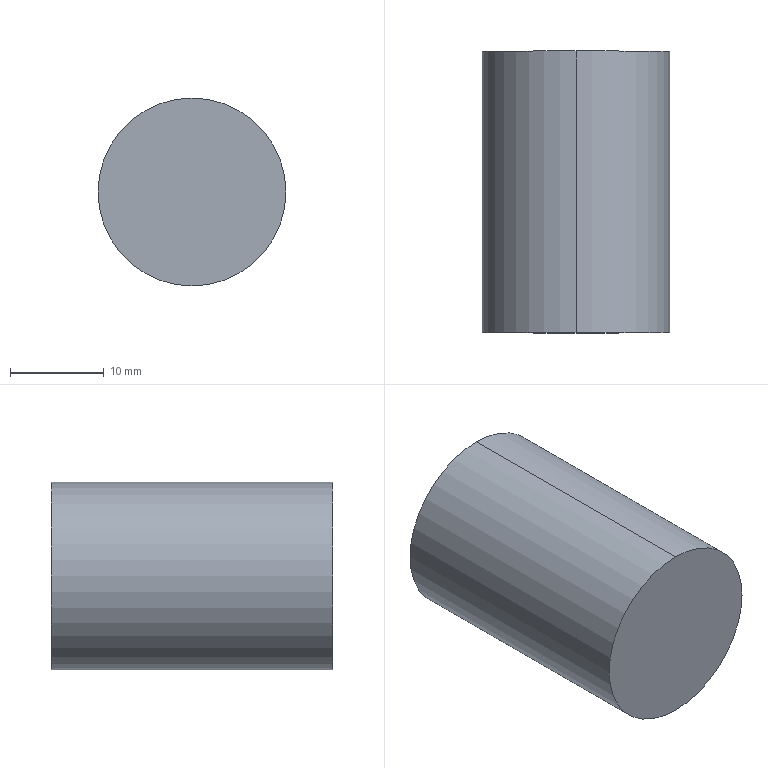Part | SolidWorks | features Extrusion 1 | 1 solid | 4 faces | box 20 x 30 x 20 mm | volume 9425 mm3 | cylinder 2 | plane 2 | commonest cylinder face diameters 20 x2
STEP:
#1=CARTESIAN_POINT('',(0.,30.,10.));
#2=VERTEX_POINT('',#1);
#3=CARTESIAN_POINT('',(0.,30.,-10.));
#4=VERTEX_POINT('',#3);
#5=CARTESIAN_POINT('',(0.,30.,0.));
#6=DIRECTION('',(0.,1.,0.));
#7=DIRECTION('',(0.,0.,1.));
#8=AXIS2_PLACEMENT_3D('',#5,#6,#7);
#9=CIRCLE('',#8,10.);
#10=EDGE_CURVE('',#2,#4,#9,.T.);
#11=ORIENTED_EDGE('',*,*,#10,.F.);
#12=CARTESIAN_POINT('',(0.,0.,10.));
#13=VERTEX_POINT('',#12);
#14=CARTESIAN_POINT('',(0.,30.,10.));
#15=DIRECTION('',(0.,-1.,0.));
#16=VECTOR('',#15,1000.);
#17=LINE('',#14,#16);
#18=EDGE_CURVE('',#2,#13,#17,.T.);
#19=ORIENTED_EDGE('',*,*,#18,.T.);
#20=CARTESIAN_POINT('',(0.,0.,-10.));
#21=VERTEX_POINT('',#20);
#22=CARTESIAN_POINT('',(0.,0.,0.));
#23=DIRECTION('',(0.,1.,0.));
#24=DIRECTION('',(0.,0.,1.));
#25=AXIS2_PLACEMENT_3D('',#22,#23,#24);
#26=CIRCLE('',#25,10.);
#27=EDGE_CURVE('',#13,#21,#26,.T.);
#28=ORIENTED_EDGE('',*,*,#27,.T.);
#29=CARTESIAN_POINT('',(0.,30.,-10.));
#30=DIRECTION('',(0.,-1.,0.));
#31=VECTOR('',#30,1000.);
#32=LINE('',#29,#31);
#33=EDGE_CURVE('',#4,#21,#32,.T.);
#34=ORIENTED_EDGE('',*,*,#33,.F.);
#35=EDGE_LOOP('',(#11,#19,#28,#34));
#36=FACE_OUTER_BOUND('',#35,.T.);
#37=CARTESIAN_POINT('',(0.,30.,0.));
#38=DIRECTION('',(0.,-1.,0.));
#39=DIRECTION('',(0.,0.,-1.));
#40=AXIS2_PLACEMENT_3D('',#37,#38,#39);
#41=CYLINDRICAL_SURFACE('',#40,10.);
#42=ADVANCED_FACE('',(#36),#41,.T.);
#43=ORIENTED_EDGE('',*,*,#18,.F.);
#44=CARTESIAN_POINT('',(0.,30.,0.));
#45=DIRECTION('',(0.,1.,0.));
#46=DIRECTION('',(0.,0.,1.));
#47=AXIS2_PLACEMENT_3D('',#44,#45,#46);
#48=CIRCLE('',#47,10.);
#49=EDGE_CURVE('',#4,#2,#48,.T.);
#50=ORIENTED_EDGE('',*,*,#49,.F.);
#51=ORIENTED_EDGE('',*,*,#33,.T.);
#52=CARTESIAN_POINT('',(0.,0.,0.));
#53=DIRECTION('',(0.,1.,0.));
#54=DIRECTION('',(0.,0.,1.));
#55=AXIS2_PLACEMENT_3D('',#52,#53,#54);
#56=CIRCLE('',#55,10.);
#57=EDGE_CURVE('',#21,#13,#56,.T.);
#58=ORIENTED_EDGE('',*,*,#57,.T.);
#59=EDGE_LOOP('',(#43,#50,#51,#58));
#60=FACE_OUTER_BOUND('',#59,.T.);
#61=CARTESIAN_POINT('',(0.,30.,0.));
#62=DIRECTION('',(0.,-1.,0.));
#63=DIRECTION('',(0.,0.,-1.));
#64=AXIS2_PLACEMENT_3D('',#61,#62,#63);
#65=CYLINDRICAL_SURFACE('',#64,10.);
#66=ADVANCED_FACE('',(#60),#65,.T.);
#67=ORIENTED_EDGE('',*,*,#49,.T.);
#68=ORIENTED_EDGE('',*,*,#10,.T.);
#69=EDGE_LOOP('',(#67,#68));
#70=FACE_OUTER_BOUND('',#69,.T.);
#71=CARTESIAN_POINT('',(0.,30.,0.));
#72=DIRECTION('',(0.,1.,0.));
#73=DIRECTION('',(0.,0.,1.));
#74=AXIS2_PLACEMENT_3D('',#71,#72,#73);
#75=PLANE('',#74);
#76=ADVANCED_FACE('',(#70),#75,.T.);
#77=ORIENTED_EDGE('',*,*,#57,.F.);
#78=ORIENTED_EDGE('',*,*,#27,.F.);
#79=EDGE_LOOP('',(#77,#78));
#80=FACE_OUTER_BOUND('',#79,.T.);
#81=CARTESIAN_POINT('',(0.,0.,0.));
#82=DIRECTION('',(0.,1.,0.));
#83=DIRECTION('',(0.,0.,1.));
#84=AXIS2_PLACEMENT_3D('',#81,#82,#83);
#85=PLANE('',#84);
#86=ADVANCED_FACE('',(#80),#85,.F.);
#87=CLOSED_SHELL('',(#42,#66,#76,#86));
#88=MANIFOLD_SOLID_BREP('',#87);
#89=CARTESIAN_POINT('',(0.,0.,0.));
#90=DIRECTION('',(0.,0.,1.));
#91=DIRECTION('',(1.,0.,0.));
#92=AXIS2_PLACEMENT_3D('',#89,#90,#91);
#93=(LENGTH_UNIT()NAMED_UNIT(*)SI_UNIT(.MILLI.,.METRE.));
#94=UNCERTAINTY_MEASURE_WITH_UNIT(LENGTH_MEASURE(0.00001),#93,'','');
#95=(NAMED_UNIT(*)PLANE_ANGLE_UNIT()SI_UNIT($,.RADIAN.));
#96=(NAMED_UNIT(*)SI_UNIT($,.STERADIAN.)SOLID_ANGLE_UNIT());
#97=(GEOMETRIC_REPRESENTATION_CONTEXT(3)GLOBAL_UNCERTAINTY_ASSIGNED_CONTEXT((#94))GLOBAL_UNIT_ASSIGNED_CONTEXT((#93,#95,#96))REPRESENTATION_CONTEXT('',''));
#98=ADVANCED_BREP_SHAPE_REPRESENTATION('',(#88,#92),#97);